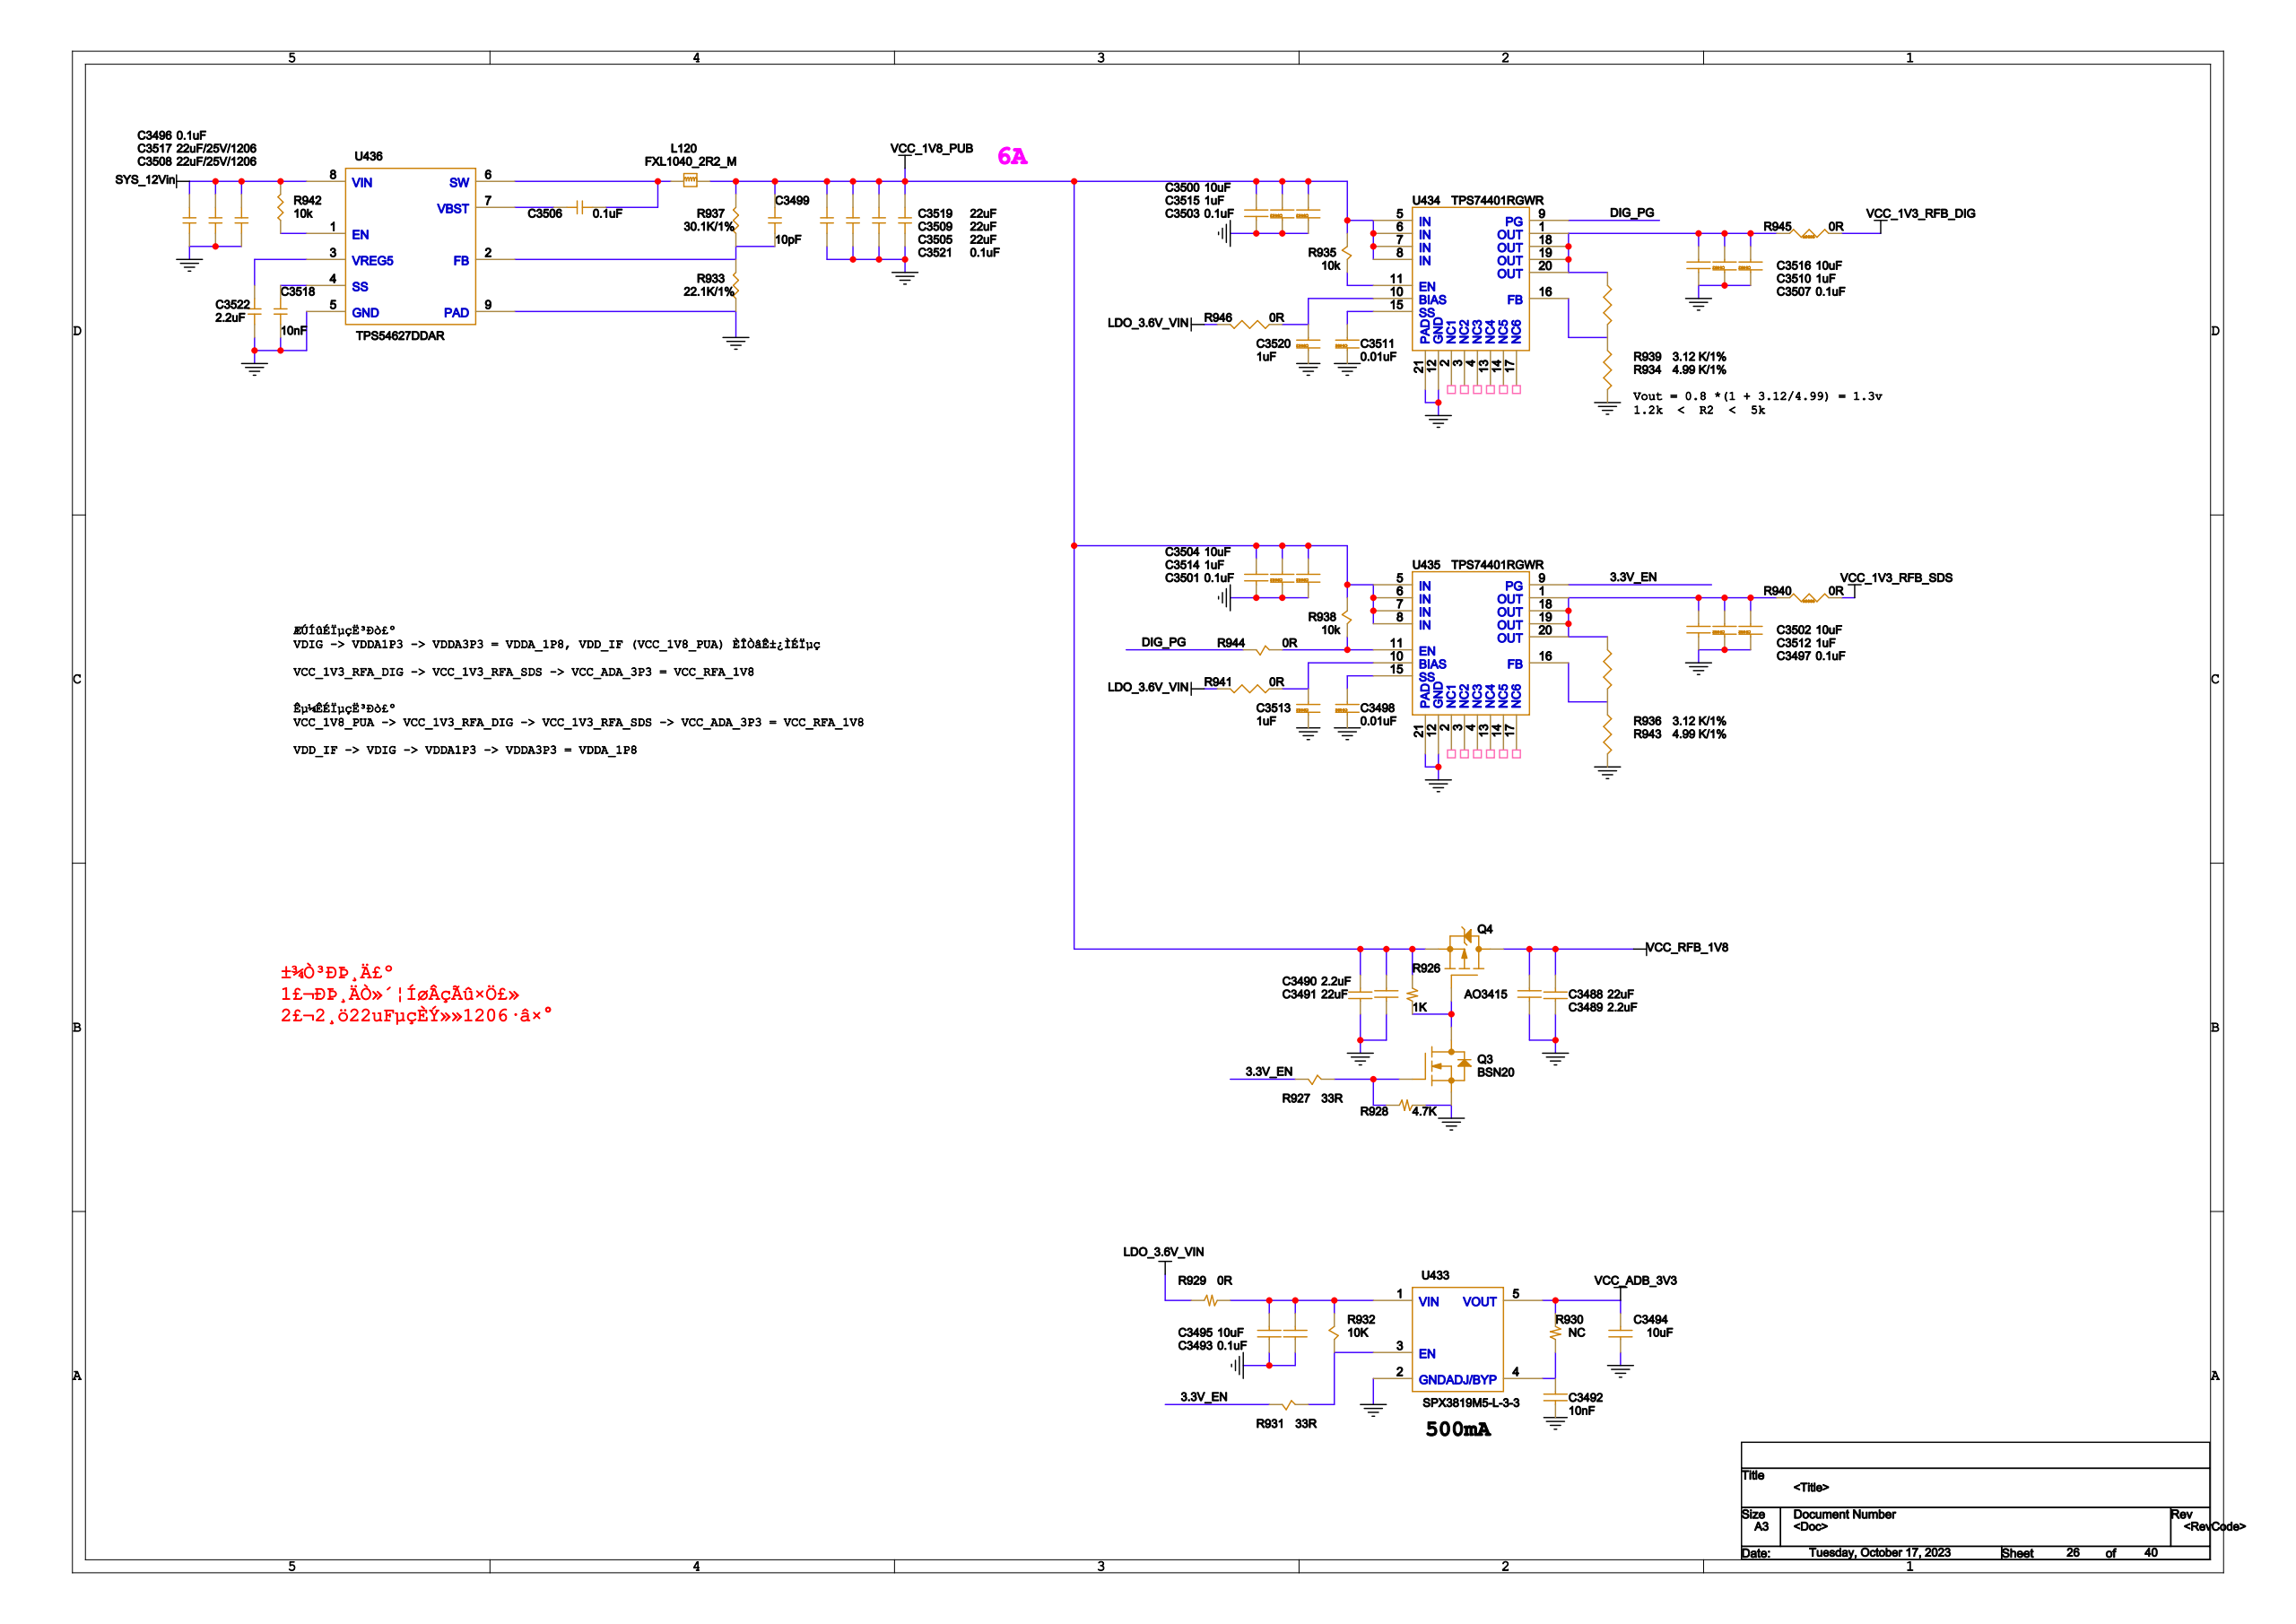Circuit board | Cadence Allegro | 1793 parts | 1223 nets | one sheet of the schematic
Parts on this sheet (reference | value | footprint):
C3488 | 22uF | C0603
C3489 | 2.2uF | C0402
C3490 | 2.2uF | C0402
C3491 | 22uF | C0603
C3492 | 10nF | C0402
C3493 | 0.1uF | C0402
C3494 | 10uF | C0402
C3495 | 10uF | C0402
C3496 | 0.1uF | C0402
C3497 | 0.1uF | C0402
C3498 | 0.01uF | C0402
C3499 | 10pF | C0402
C3500 | 10uF | C0402
C3501 | 0.1uF | C0402
C3502 | 10uF | C0402
C3503 | 0.1uF | C0402
C3504 | 10uF | C0402
C3505 | 22uF | C0603
C3506 | 0.1uF | C0402
C3507 | 0.1uF | C0402
C3508 | 22uF/25V/1206 | 1206
C3509 | 22uF | C0603
C3510 | 1uF | C0402
C3511 | 0.01uF | C0402
C3512 | 1uF | C0402
C3513 | 1uF | C0402
C3514 | 1uF | C0402
C3515 | 1uF | C0402
C3516 | 10uF | C0402
C3517 | 22uF/25V/1206 | 1206
C3518 | 10nF | C0402
C3519 | 22uF | C0603
C3520 | 1uF | C0402
C3521 | 0.1uF | C0402
C3522 | 2.2uF | C0402
L120 | FXL1040_2R2_M | SMD_11_5X10
Q3 | BSN20 | SOT23
Q4 | AO3415 | SOT23
R926 | 1K | R0402
R927 | 33R | R0402
R928 | 4.7K | R0402
R929 | 0R | R0402
R930 | NC | R0402
R931 | 33R | R0402
R932 | 10K | R0402
R933 | 22.1K/1% | R0402
R934 | 4.99 K/1% | R0402
R935 | 10K | R0402
R936 | 3.12 K/1% | R0402
R937 | 30.1K/1% | R0402
R938 | 10K | R0402
R939 | 3.12 K/1% | R0402
R940 | 0R | R0805
R941 | 0R | R0402
R942 | 10k | R0402
R943 | 4.99 K/1% | R0402
R944 | 0R | R0402
R945 | 0R | R0805
R946 | 0R | R0402
U433 | SPX3819M5-L-3-3 | SOT-23-5
U434 | TPS74401RGWR | TPS74401RGWR_VQFN
U435 | TPS74401RGWR | TPS74401RGWR_VQFN
U436 | TPS54627DDAR | POWER-SO8
Nets of these parts (net: part-pin ...):
GND: C3488-2 C3489-1 C3490-1 C3491-2 C3492-2 C3493-1 C3494-1 C3495-1 C3496-1 C3497-1 C3498-1 C3500-2 C3501-1 C3502-2 C3503-1 C3504-2 C3505-1 C3507-1 C3508-1 C3509-1 C3510-1 C3511-1 C3512-1 C3513-1 C3514-1 C3515-1 C3516-2 C3517-1 C3518-1 C3519-1 C3520-1 C3521-1 C3522-1 Q3-2 R928-2 R933-2 R934-2 R943-2 U433-2 U434-12 U434-21 U435-12 U435-21 U436-5 U436-9
SYS_12VIN: C3496-2 C3508-2 C3517-2 R942-1 U436-8
LDO_3.6V_VIN: R929-1 R941-2 R946-2
N17266051: R942-2 U436-1
VCC_1V3_RFB_DIG: R945-2
VCC_1V3_RFB_SDS: R940-2
VCC_RFB_1V8: C3488-1 C3489-2 Q4-3
VCC_1V8_PUB: C3490-2 C3491-1 C3499-2 C3500-1 C3501-2 C3503-2 C3504-1 C3505-2 C3509-2 C3514-2 C3515-2 C3519-2 C3521-2 L120-2 Q4-2 R926-1 R935-2 R937-1 R938-2 U434-5 U434-6 U434-7 U434-8 U435-5 U435-6 U435-7 U435-8
N17266091: C3518-2 U436-4
N17266149: C3497-2 C3502-1 C3512-2 R936-1 R940-1 U435-1 U435-18 U435-19 U435-20
N17265943: C3507-2 C3510-2 C3516-1 R939-1 R945-1 U434-1 U434-18 U434-19 U434-20
VCC_ADB_3V3: C3494-2 R930-1 U433-5
N17264625: C3493-2 C3495-2 R929-2 R932-2 U433-1
N17266071: C3522-2 U436-3
N17266017: C3506-2 L120-1 U436-6
N17266059: C3499-1 R933-1 R937-2 U436-2
N17266047: C3506-1 U436-7
N17265996: C3520-2 R946-1 U434-10
N17265967: R935-1 U434-11
N17265979: R934-1 R939-2 U434-16
DIG_PG_17265938: R944-2 U434-9
N17265981: C3511-2 U434-15
N17266181: C3513-2 R941-1 U435-10
N17266169: R938-1 R944-1 U435-11
N17266185: R936-2 R943-1 U435-16
3.3V_EN_17262149: R927-2 R931-2 U435-9
N17266187: C3498-2 U435-15
N17264648: C3492-1 R930-2 U433-4
N17262132: Q3-3 Q4-1 R926-2
N17262152: Q3-1 R927-1 R928-1
N17264643: R931-1 R932-1 U433-3